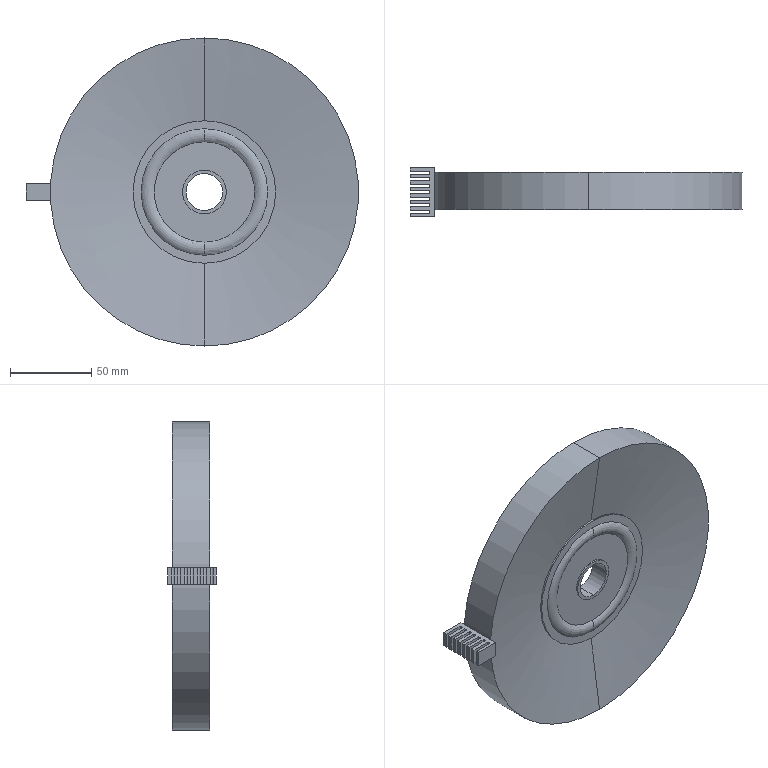Part | SolidWorks | features ICE 1, MBimport 1 | 5 solids | 80 faces | box 205 x 30 x 190 mm | volume 425990 mm3 | plane 41 | cylinder 27 | torus 8 | cone 4 | commonest cylinder face diameters 24.8 x8 2.576 x7 27 x4 88 x4 22.8 x2 190 x2